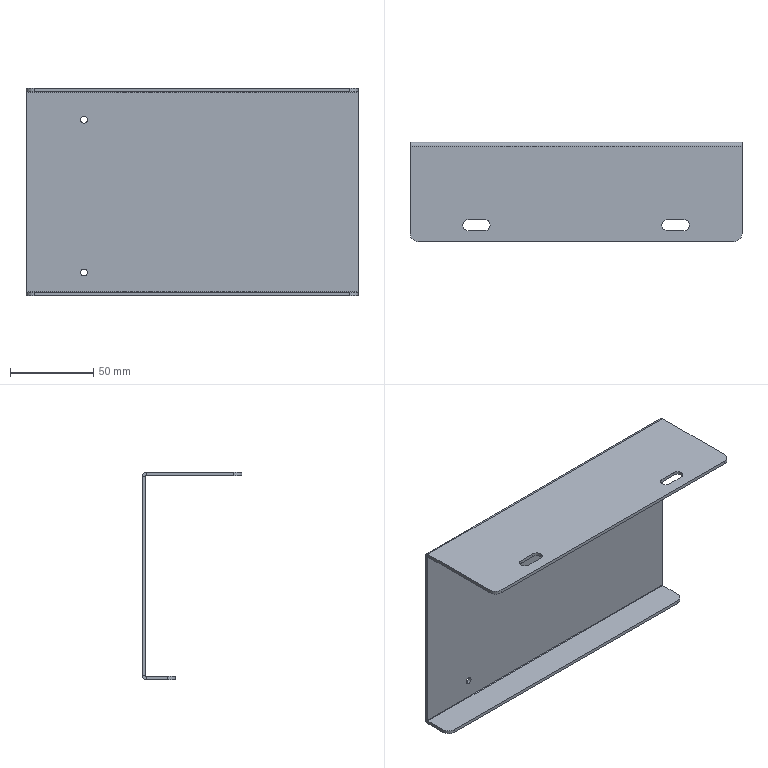Part | SolidWorks | features Fillet 1, FlatPattern 1, HoleWzd 1, ICE 1, SMBaseFlange 1, SheetMetal 1 | 1 solid | 40 faces | box 200 x 60 x 125 mm | volume 79463 mm3 | plane 22 | cylinder 18 | commonest cylinder face diameters 6.5 x6 4.2 x4 10 x4 0.6 x2 4.6 x2
STEP:
#1=CARTESIAN_POINT('',(35.,-2.,-113.1));
#2=VERTEX_POINT('',#1);
#3=CARTESIAN_POINT('',(35.,-2.,-108.9));
#4=VERTEX_POINT('',#3);
#5=CARTESIAN_POINT('',(35.,-2.,-111.));
#6=DIRECTION('',(0.,1.,0.));
#7=DIRECTION('',(0.,0.,1.));
#8=AXIS2_PLACEMENT_3D('',#5,#6,#7);
#9=CIRCLE('',#8,2.1);
#10=EDGE_CURVE('',#2,#4,#9,.T.);
#11=ORIENTED_EDGE('',*,*,#10,.F.);
#12=CARTESIAN_POINT('',(35.,0.,-113.1));
#13=VERTEX_POINT('',#12);
#14=CARTESIAN_POINT('',(35.,0.,-113.1));
#15=DIRECTION('',(0.,1.,0.));
#16=VECTOR('',#15,1000.);
#17=LINE('',#14,#16);
#18=EDGE_CURVE('',#2,#13,#17,.T.);
#19=ORIENTED_EDGE('',*,*,#18,.T.);
#20=CARTESIAN_POINT('',(35.,0.,-108.9));
#21=VERTEX_POINT('',#20);
#22=CARTESIAN_POINT('',(35.,0.,-111.));
#23=DIRECTION('',(0.,1.,0.));
#24=DIRECTION('',(0.,0.,1.));
#25=AXIS2_PLACEMENT_3D('',#22,#23,#24);
#26=CIRCLE('',#25,2.1);
#27=EDGE_CURVE('',#13,#21,#26,.T.);
#28=ORIENTED_EDGE('',*,*,#27,.T.);
#29=CARTESIAN_POINT('',(35.,0.,-108.9));
#30=DIRECTION('',(0.,1.,0.));
#31=VECTOR('',#30,1000.);
#32=LINE('',#29,#31);
#33=EDGE_CURVE('',#4,#21,#32,.T.);
#34=ORIENTED_EDGE('',*,*,#33,.F.);
#35=EDGE_LOOP('',(#11,#19,#28,#34));
#36=FACE_OUTER_BOUND('',#35,.T.);
#37=CARTESIAN_POINT('',(35.,0.,-111.));
#38=DIRECTION('',(0.,1.,0.));
#39=DIRECTION('',(0.,0.,1.));
#40=AXIS2_PLACEMENT_3D('',#37,#38,#39);
#41=CYLINDRICAL_SURFACE('',#40,2.1);
#42=ADVANCED_FACE('',(#36),#41,.F.);
#43=CARTESIAN_POINT('',(35.,-2.,-21.1));
#44=VERTEX_POINT('',#43);
#45=CARTESIAN_POINT('',(35.,-2.,-16.9));
#46=VERTEX_POINT('',#45);
#47=CARTESIAN_POINT('',(35.,-2.,-19.));
#48=DIRECTION('',(0.,1.,0.));
#49=DIRECTION('',(0.,0.,1.));
#50=AXIS2_PLACEMENT_3D('',#47,#48,#49);
#51=CIRCLE('',#50,2.1);
#52=EDGE_CURVE('',#44,#46,#51,.T.);
#53=ORIENTED_EDGE('',*,*,#52,.F.);
#54=CARTESIAN_POINT('',(35.,0.,-21.1));
#55=VERTEX_POINT('',#54);
#56=CARTESIAN_POINT('',(35.,0.,-21.1));
#57=DIRECTION('',(0.,1.,0.));
#58=VECTOR('',#57,1000.);
#59=LINE('',#56,#58);
#60=EDGE_CURVE('',#44,#55,#59,.T.);
#61=ORIENTED_EDGE('',*,*,#60,.T.);
#62=CARTESIAN_POINT('',(35.,0.,-16.9));
#63=VERTEX_POINT('',#62);
#64=CARTESIAN_POINT('',(35.,0.,-19.));
#65=DIRECTION('',(0.,1.,0.));
#66=DIRECTION('',(0.,0.,1.));
#67=AXIS2_PLACEMENT_3D('',#64,#65,#66);
#68=CIRCLE('',#67,2.1);
#69=EDGE_CURVE('',#55,#63,#68,.T.);
#70=ORIENTED_EDGE('',*,*,#69,.T.);
#71=CARTESIAN_POINT('',(35.,0.,-16.9));
#72=DIRECTION('',(0.,1.,0.));
#73=VECTOR('',#72,1000.);
#74=LINE('',#71,#73);
#75=EDGE_CURVE('',#46,#63,#74,.T.);
#76=ORIENTED_EDGE('',*,*,#75,.F.);
#77=EDGE_LOOP('',(#53,#61,#70,#76));
#78=FACE_OUTER_BOUND('',#77,.T.);
#79=CARTESIAN_POINT('',(35.,0.,-19.));
#80=DIRECTION('',(0.,1.,0.));
#81=DIRECTION('',(0.,0.,1.));
#82=AXIS2_PLACEMENT_3D('',#79,#80,#81);
#83=CYLINDRICAL_SURFACE('',#82,2.1);
#84=ADVANCED_FACE('',(#78),#83,.F.);
#85=CARTESIAN_POINT('',(165.,-46.75,-2.));
#86=VERTEX_POINT('',#85);
#87=CARTESIAN_POINT('',(168.25,-50.,-2.));
#88=VERTEX_POINT('',#87);
#89=CARTESIAN_POINT('',(165.,-50.,-2.));
#90=DIRECTION('',(0.,0.,-1.));
#91=DIRECTION('',(0.,-1.,0.));
#92=AXIS2_PLACEMENT_3D('',#89,#90,#91);
#93=CIRCLE('',#92,3.25);
#94=EDGE_CURVE('',#86,#88,#93,.T.);
#95=ORIENTED_EDGE('',*,*,#94,.T.);
#96=CARTESIAN_POINT('',(168.25,-50.,0.));
#97=VERTEX_POINT('',#96);
#98=CARTESIAN_POINT('',(168.25,-50.,-10.));
#99=DIRECTION('',(0.,0.,1.));
#100=VECTOR('',#99,1000.);
#101=LINE('',#98,#100);
#102=EDGE_CURVE('',#88,#97,#101,.T.);
#103=ORIENTED_EDGE('',*,*,#102,.T.);
#104=CARTESIAN_POINT('',(165.,-46.75,0.));
#105=VERTEX_POINT('',#104);
#106=CARTESIAN_POINT('',(165.,-50.,0.));
#107=DIRECTION('',(0.,0.,-1.));
#108=DIRECTION('',(-1.,0.,0.));
#109=AXIS2_PLACEMENT_3D('',#106,#107,#108);
#110=CIRCLE('',#109,3.25);
#111=EDGE_CURVE('',#105,#97,#110,.T.);
#112=ORIENTED_EDGE('',*,*,#111,.F.);
#113=CARTESIAN_POINT('',(165.,-46.75,-10.));
#114=DIRECTION('',(0.,0.,1.));
#115=VECTOR('',#114,1000.);
#116=LINE('',#113,#115);
#117=EDGE_CURVE('',#86,#105,#116,.T.);
#118=ORIENTED_EDGE('',*,*,#117,.F.);
#119=EDGE_LOOP('',(#95,#103,#112,#118));
#120=FACE_OUTER_BOUND('',#119,.T.);
#121=CARTESIAN_POINT('',(165.,-50.,-10.));
#122=DIRECTION('',(0.,0.,1.));
#123=DIRECTION('',(1.,0.,0.));
#124=AXIS2_PLACEMENT_3D('',#121,#122,#123);
#125=CYLINDRICAL_SURFACE('',#124,3.25);
#126=ADVANCED_FACE('',(#120),#125,.F.);
#127=CARTESIAN_POINT('',(45.,-46.75,-2.));
#128=VERTEX_POINT('',#127);
#129=CARTESIAN_POINT('',(48.25,-50.,-2.));
#130=VERTEX_POINT('',#129);
#131=CARTESIAN_POINT('',(45.,-50.,-2.));
#132=DIRECTION('',(0.,0.,-1.));
#133=DIRECTION('',(0.,-1.,0.));
#134=AXIS2_PLACEMENT_3D('',#131,#132,#133);
#135=CIRCLE('',#134,3.25);
#136=EDGE_CURVE('',#128,#130,#135,.T.);
#137=ORIENTED_EDGE('',*,*,#136,.T.);
#138=CARTESIAN_POINT('',(48.25,-50.,0.));
#139=VERTEX_POINT('',#138);
#140=CARTESIAN_POINT('',(48.25,-50.,-10.));
#141=DIRECTION('',(0.,0.,1.));
#142=VECTOR('',#141,1000.);
#143=LINE('',#140,#142);
#144=EDGE_CURVE('',#130,#139,#143,.T.);
#145=ORIENTED_EDGE('',*,*,#144,.T.);
#146=CARTESIAN_POINT('',(45.,-46.75,0.));
#147=VERTEX_POINT('',#146);
#148=CARTESIAN_POINT('',(45.,-50.,0.));
#149=DIRECTION('',(0.,0.,-1.));
#150=DIRECTION('',(-1.,0.,0.));
#151=AXIS2_PLACEMENT_3D('',#148,#149,#150);
#152=CIRCLE('',#151,3.25);
#153=EDGE_CURVE('',#147,#139,#152,.T.);
#154=ORIENTED_EDGE('',*,*,#153,.F.);
#155=CARTESIAN_POINT('',(45.,-46.75,-10.));
#156=DIRECTION('',(0.,0.,1.));
#157=VECTOR('',#156,1000.);
#158=LINE('',#155,#157);
#159=EDGE_CURVE('',#128,#147,#158,.T.);
#160=ORIENTED_EDGE('',*,*,#159,.F.);
#161=EDGE_LOOP('',(#137,#145,#154,#160));
#162=FACE_OUTER_BOUND('',#161,.T.);
#163=CARTESIAN_POINT('',(45.,-50.,-10.));
#164=DIRECTION('',(0.,0.,1.));
#165=DIRECTION('',(1.,0.,0.));
#166=AXIS2_PLACEMENT_3D('',#163,#164,#165);
#167=CYLINDRICAL_SURFACE('',#166,3.25);
#168=ADVANCED_FACE('',(#162),#167,.F.);
#169=CARTESIAN_POINT('',(195.,-60.,0.));
#170=VERTEX_POINT('',#169);
#171=CARTESIAN_POINT('',(5.,-60.,0.));
#172=VERTEX_POINT('',#171);
#173=CARTESIAN_POINT('',(200.,-60.,0.));
#174=DIRECTION('',(-1.,0.,0.));
#175=VECTOR('',#174,1000.);
#176=LINE('',#173,#175);
#177=EDGE_CURVE('',#170,#172,#176,.T.);
#178=ORIENTED_EDGE('',*,*,#177,.F.);
#179=CARTESIAN_POINT('',(200.,-55.,0.));
#180=VERTEX_POINT('',#179);
#181=CARTESIAN_POINT('',(195.,-55.,0.));
#182=DIRECTION('',(0.,0.,1.));
#183=DIRECTION('',(0.,-1.,0.));
#184=AXIS2_PLACEMENT_3D('',#181,#182,#183);
#185=CIRCLE('',#184,5.);
#186=EDGE_CURVE('',#170,#180,#185,.T.);
#187=ORIENTED_EDGE('',*,*,#186,.T.);
#188=CARTESIAN_POINT('',(200.,-2.3,0.));
#189=VERTEX_POINT('',#188);
#190=CARTESIAN_POINT('',(200.,0.,0.));
#191=DIRECTION('',(0.,1.,0.));
#192=VECTOR('',#191,1000.);
#193=LINE('',#190,#192);
#194=EDGE_CURVE('',#180,#189,#193,.T.);
#195=ORIENTED_EDGE('',*,*,#194,.T.);
#196=CARTESIAN_POINT('',(0.,-2.3,0.));
#197=VERTEX_POINT('',#196);
#198=CARTESIAN_POINT('',(200.,-2.3,0.));
#199=DIRECTION('',(-1.,0.,0.));
#200=VECTOR('',#199,1000.);
#201=LINE('',#198,#200);
#202=EDGE_CURVE('',#189,#197,#201,.T.);
#203=ORIENTED_EDGE('',*,*,#202,.T.);
#204=CARTESIAN_POINT('',(0.,-55.,0.));
#205=VERTEX_POINT('',#204);
#206=CARTESIAN_POINT('',(0.,0.,0.));
#207=DIRECTION('',(0.,1.,0.));
#208=VECTOR('',#207,1000.);
#209=LINE('',#206,#208);
#210=EDGE_CURVE('',#205,#197,#209,.T.);
#211=ORIENTED_EDGE('',*,*,#210,.F.);
#212=CARTESIAN_POINT('',(5.,-55.,0.));
#213=DIRECTION('',(0.,0.,1.));
#214=DIRECTION('',(0.,-1.,0.));
#215=AXIS2_PLACEMENT_3D('',#212,#213,#214);
#216=CIRCLE('',#215,5.);
#217=EDGE_CURVE('',#205,#172,#216,.T.);
#218=ORIENTED_EDGE('',*,*,#217,.T.);
#219=EDGE_LOOP('',(#178,#187,#195,#203,#211,#218));
#220=FACE_OUTER_BOUND('',#219,.T.);
#221=CARTESIAN_POINT('',(35.,-46.75,0.));
#222=VERTEX_POINT('',#221);
#223=CARTESIAN_POINT('',(45.,-46.75,0.));
#224=DIRECTION('',(1.,0.,0.));
#225=VECTOR('',#224,1000.);
#226=LINE('',#223,#225);
#227=EDGE_CURVE('',#222,#147,#226,.T.);
#228=ORIENTED_EDGE('',*,*,#227,.T.);
#229=ORIENTED_EDGE('',*,*,#153,.T.);
#230=CARTESIAN_POINT('',(45.,-53.25,0.));
#231=VERTEX_POINT('',#230);
#232=CARTESIAN_POINT('',(45.,-50.,0.));
#233=DIRECTION('',(0.,0.,-1.));
#234=DIRECTION('',(-1.,0.,0.));
#235=AXIS2_PLACEMENT_3D('',#232,#233,#234);
#236=CIRCLE('',#235,3.25);
#237=EDGE_CURVE('',#139,#231,#236,.T.);
#238=ORIENTED_EDGE('',*,*,#237,.T.);
#239=CARTESIAN_POINT('',(35.,-53.25,0.));
#240=VERTEX_POINT('',#239);
#241=CARTESIAN_POINT('',(45.,-53.25,0.));
#242=DIRECTION('',(-1.,0.,0.));
#243=VECTOR('',#242,1000.);
#244=LINE('',#241,#243);
#245=EDGE_CURVE('',#231,#240,#244,.T.);
#246=ORIENTED_EDGE('',*,*,#245,.T.);
#247=CARTESIAN_POINT('',(35.,-50.,0.));
#248=DIRECTION('',(0.,0.,-1.));
#249=DIRECTION('',(-1.,0.,0.));
#250=AXIS2_PLACEMENT_3D('',#247,#248,#249);
#251=CIRCLE('',#250,3.25);
#252=EDGE_CURVE('',#240,#222,#251,.T.);
#253=ORIENTED_EDGE('',*,*,#252,.T.);
#254=EDGE_LOOP('',(#228,#229,#238,#246,#253));
#255=FACE_BOUND('',#254,.T.);
#256=CARTESIAN_POINT('',(155.,-46.75,0.));
#257=VERTEX_POINT('',#256);
#258=CARTESIAN_POINT('',(165.,-46.75,0.));
#259=DIRECTION('',(1.,0.,0.));
#260=VECTOR('',#259,1000.);
#261=LINE('',#258,#260);
#262=EDGE_CURVE('',#257,#105,#261,.T.);
#263=ORIENTED_EDGE('',*,*,#262,.T.);
#264=ORIENTED_EDGE('',*,*,#111,.T.);
#265=CARTESIAN_POINT('',(165.,-53.25,0.));
#266=VERTEX_POINT('',#265);
#267=CARTESIAN_POINT('',(165.,-50.,0.));
#268=DIRECTION('',(0.,0.,-1.));
#269=DIRECTION('',(-1.,0.,0.));
#270=AXIS2_PLACEMENT_3D('',#267,#268,#269);
#271=CIRCLE('',#270,3.25);
#272=EDGE_CURVE('',#97,#266,#271,.T.);
#273=ORIENTED_EDGE('',*,*,#272,.T.);
#274=CARTESIAN_POINT('',(155.,-53.25,0.));
#275=VERTEX_POINT('',#274);
#276=CARTESIAN_POINT('',(165.,-53.25,0.));
#277=DIRECTION('',(-1.,0.,0.));
#278=VECTOR('',#277,1000.);
#279=LINE('',#276,#278);
#280=EDGE_CURVE('',#266,#275,#279,.T.);
#281=ORIENTED_EDGE('',*,*,#280,.T.);
#282=CARTESIAN_POINT('',(155.,-50.,0.));
#283=DIRECTION('',(0.,0.,-1.));
#284=DIRECTION('',(-1.,0.,0.));
#285=AXIS2_PLACEMENT_3D('',#282,#283,#284);
#286=CIRCLE('',#285,3.25);
#287=EDGE_CURVE('',#275,#257,#286,.T.);
#288=ORIENTED_EDGE('',*,*,#287,.T.);
#289=EDGE_LOOP('',(#263,#264,#273,#281,#288));
#290=FACE_BOUND('',#289,.T.);
#291=CARTESIAN_POINT('',(200.,0.,0.));
#292=DIRECTION('',(0.,0.,1.));
#293=DIRECTION('',(0.,-1.,0.));
#294=AXIS2_PLACEMENT_3D('',#291,#292,#293);
#295=PLANE('',#294);
#296=ADVANCED_FACE('',(#220,#255,#290),#295,.T.);
#297=ORIENTED_EDGE('',*,*,#136,.F.);
#298=CARTESIAN_POINT('',(35.,-46.75,-2.));
#299=VERTEX_POINT('',#298);
#300=CARTESIAN_POINT('',(200.,-46.75,-2.));
#301=DIRECTION('',(1.,0.,0.));
#302=VECTOR('',#301,1000.);
#303=LINE('',#300,#302);
#304=EDGE_CURVE('',#299,#128,#303,.T.);
#305=ORIENTED_EDGE('',*,*,#304,.F.);
#306=CARTESIAN_POINT('',(35.,-53.25,-2.));
#307=VERTEX_POINT('',#306);
#308=CARTESIAN_POINT('',(35.,-50.,-2.));
#309=DIRECTION('',(0.,0.,-1.));
#310=DIRECTION('',(0.,-1.,0.));
#311=AXIS2_PLACEMENT_3D('',#308,#309,#310);
#312=CIRCLE('',#311,3.25);
#313=EDGE_CURVE('',#307,#299,#312,.T.);
#314=ORIENTED_EDGE('',*,*,#313,.F.);
#315=CARTESIAN_POINT('',(45.,-53.25,-2.));
#316=VERTEX_POINT('',#315);
#317=CARTESIAN_POINT('',(200.,-53.25,-2.));
#318=DIRECTION('',(-1.,0.,0.));
#319=VECTOR('',#318,1000.);
#320=LINE('',#317,#319);
#321=EDGE_CURVE('',#316,#307,#320,.T.);
#322=ORIENTED_EDGE('',*,*,#321,.F.);
#323=CARTESIAN_POINT('',(45.,-50.,-2.));
#324=DIRECTION('',(0.,0.,-1.));
#325=DIRECTION('',(0.,-1.,0.));
#326=AXIS2_PLACEMENT_3D('',#323,#324,#325);
#327=CIRCLE('',#326,3.25);
#328=EDGE_CURVE('',#130,#316,#327,.T.);
#329=ORIENTED_EDGE('',*,*,#328,.F.);
#330=EDGE_LOOP('',(#297,#305,#314,#322,#329));
#331=FACE_BOUND('',#330,.T.);
#332=CARTESIAN_POINT('',(200.,-55.,-2.));
#333=VERTEX_POINT('',#332);
#334=CARTESIAN_POINT('',(200.,-2.3,-2.));
#335=VERTEX_POINT('',#334);
#336=CARTESIAN_POINT('',(200.,0.,-2.));
#337=DIRECTION('',(0.,1.,0.));
#338=VECTOR('',#337,1000.);
#339=LINE('',#336,#338);
#340=EDGE_CURVE('',#333,#335,#339,.T.);
#341=ORIENTED_EDGE('',*,*,#340,.F.);
#342=CARTESIAN_POINT('',(195.,-60.,-2.));
#343=VERTEX_POINT('',#342);
#344=CARTESIAN_POINT('',(195.,-55.,-2.));
#345=DIRECTION('',(0.,0.,-1.));
#346=DIRECTION('',(0.,-1.,0.));
#347=AXIS2_PLACEMENT_3D('',#344,#345,#346);
#348=CIRCLE('',#347,5.);
#349=EDGE_CURVE('',#333,#343,#348,.T.);
#350=ORIENTED_EDGE('',*,*,#349,.T.);
#351=CARTESIAN_POINT('',(5.,-60.,-2.));
#352=VERTEX_POINT('',#351);
#353=CARTESIAN_POINT('',(200.,-60.,-2.));
#354=DIRECTION('',(-1.,0.,0.));
#355=VECTOR('',#354,1000.);
#356=LINE('',#353,#355);
#357=EDGE_CURVE('',#343,#352,#356,.T.);
#358=ORIENTED_EDGE('',*,*,#357,.T.);
#359=CARTESIAN_POINT('',(0.,-55.,-2.));
#360=VERTEX_POINT('',#359);
#361=CARTESIAN_POINT('',(5.,-55.,-2.));
#362=DIRECTION('',(0.,0.,-1.));
#363=DIRECTION('',(0.,-1.,0.));
#364=AXIS2_PLACEMENT_3D('',#361,#362,#363);
#365=CIRCLE('',#364,5.);
#366=EDGE_CURVE('',#352,#360,#365,.T.);
#367=ORIENTED_EDGE('',*,*,#366,.T.);
#368=CARTESIAN_POINT('',(0.,-2.3,-2.));
#369=VERTEX_POINT('',#368);
#370=CARTESIAN_POINT('',(0.,0.,-2.));
#371=DIRECTION('',(0.,1.,0.));
#372=VECTOR('',#371,1000.);
#373=LINE('',#370,#372);
#374=EDGE_CURVE('',#360,#369,#373,.T.);
#375=ORIENTED_EDGE('',*,*,#374,.T.);
#376=CARTESIAN_POINT('',(200.,-2.3,-2.));
#377=DIRECTION('',(-1.,0.,0.));
#378=VECTOR('',#377,1000.);
#379=LINE('',#376,#378);
#380=EDGE_CURVE('',#335,#369,#379,.T.);
#381=ORIENTED_EDGE('',*,*,#380,.F.);
#382=EDGE_LOOP('',(#341,#350,#358,#367,#375,#381));
#383=FACE_OUTER_BOUND('',#382,.T.);
#384=ORIENTED_EDGE('',*,*,#94,.F.);
#385=CARTESIAN_POINT('',(155.,-46.75,-2.));
#386=VERTEX_POINT('',#385);
#387=CARTESIAN_POINT('',(200.,-46.75,-2.));
#388=DIRECTION('',(1.,0.,0.));
#389=VECTOR('',#388,1000.);
#390=LINE('',#387,#389);
#391=EDGE_CURVE('',#386,#86,#390,.T.);
#392=ORIENTED_EDGE('',*,*,#391,.F.);
#393=CARTESIAN_POINT('',(155.,-53.25,-2.));
#394=VERTEX_POINT('',#393);
#395=CARTESIAN_POINT('',(155.,-50.,-2.));
#396=DIRECTION('',(0.,0.,-1.));
#397=DIRECTION('',(0.,-1.,0.));
#398=AXIS2_PLACEMENT_3D('',#395,#396,#397);
#399=CIRCLE('',#398,3.25);
#400=EDGE_CURVE('',#394,#386,#399,.T.);
#401=ORIENTED_EDGE('',*,*,#400,.F.);
#402=CARTESIAN_POINT('',(165.,-53.25,-2.));
#403=VERTEX_POINT('',#402);
#404=CARTESIAN_POINT('',(200.,-53.25,-2.));
#405=DIRECTION('',(-1.,0.,0.));
#406=VECTOR('',#405,1000.);
#407=LINE('',#404,#406);
#408=EDGE_CURVE('',#403,#394,#407,.T.);
#409=ORIENTED_EDGE('',*,*,#408,.F.);
#410=CARTESIAN_POINT('',(165.,-50.,-2.));
#411=DIRECTION('',(0.,0.,-1.));
#412=DIRECTION('',(0.,-1.,0.));
#413=AXIS2_PLACEMENT_3D('',#410,#411,#412);
#414=CIRCLE('',#413,3.25);
#415=EDGE_CURVE('',#88,#403,#414,.T.);
#416=ORIENTED_EDGE('',*,*,#415,.F.);
#417=EDGE_LOOP('',(#384,#392,#401,#409,#416));
#418=FACE_BOUND('',#417,.T.);
#419=CARTESIAN_POINT('',(200.,0.,-2.));
#420=DIRECTION('',(0.,0.,1.));
#421=DIRECTION('',(0.,-1.,0.));
#422=AXIS2_PLACEMENT_3D('',#419,#420,#421);
#423=PLANE('',#422);
#424=ADVANCED_FACE('',(#331,#383,#418),#423,.F.);
#425=CARTESIAN_POINT('',(200.,0.,-2.3));
#426=VERTEX_POINT('',#425);
#427=CARTESIAN_POINT('',(200.,-2.,-2.3));
#428=VERTEX_POINT('',#427);
#429=CARTESIAN_POINT('',(200.,0.,-2.3));
#430=DIRECTION('',(0.,-1.,0.));
#431=VECTOR('',#430,1000.);
#432=LINE('',#429,#431);
#433=EDGE_CURVE('',#426,#428,#432,.T.);
#434=ORIENTED_EDGE('',*,*,#433,.F.);
#435=CARTESIAN_POINT('',(200.,-2.3,-2.3));
#436=DIRECTION('',(-1.,0.,0.));
#437=DIRECTION('',(0.,0.,-1.));
#438=AXIS2_PLACEMENT_3D('',#435,#436,#437);
#439=CIRCLE('',#438,2.3);
#440=EDGE_CURVE('',#189,#426,#439,.T.);
#441=ORIENTED_EDGE('',*,*,#440,.F.);
#442=CARTESIAN_POINT('',(200.,-2.3,-2.));
#443=DIRECTION('',(0.,0.,1.));
#444=VECTOR('',#443,1000.);
#445=LINE('',#442,#444);
#446=EDGE_CURVE('',#335,#189,#445,.T.);
#447=ORIENTED_EDGE('',*,*,#446,.F.);
#448=CARTESIAN_POINT('',(200.,-2.3,-2.3));
#449=DIRECTION('',(-1.,0.,0.));
#450=DIRECTION('',(0.,0.,-1.));
#451=AXIS2_PLACEMENT_3D('',#448,#449,#450);
#452=CIRCLE('',#451,0.3);
#453=EDGE_CURVE('',#335,#428,#452,.T.);
#454=ORIENTED_EDGE('',*,*,#453,.T.);
#455=EDGE_LOOP('',(#434,#441,#447,#454));
#456=FACE_OUTER_BOUND('',#455,.T.);
#457=CARTESIAN_POINT('',(200.,0.,-2.3));
#458=DIRECTION('',(1.,0.,0.));
#459=DIRECTION('',(0.,0.,-1.));
#460=AXIS2_PLACEMENT_3D('',#457,#458,#459);
#461=PLANE('',#460);
#462=ADVANCED_FACE('',(#456),#461,.T.);
#463=CARTESIAN_POINT('',(200.,0.,-122.7));
#464=VERTEX_POINT('',#463);
#465=CARTESIAN_POINT('',(200.,0.,0.));
#466=DIRECTION('',(0.,0.,-1.));
#467=VECTOR('',#466,1000.);
#468=LINE('',#465,#467);
#469=EDGE_CURVE('',#426,#464,#468,.T.);
#470=ORIENTED_EDGE('',*,*,#469,.F.);
#471=ORIENTED_EDGE('',*,*,#433,.T.);
#472=CARTESIAN_POINT('',(200.,-2.,-122.7));
#473=VERTEX_POINT('',#472);
#474=CARTESIAN_POINT('',(200.,-2.,0.));
#475=DIRECTION('',(0.,0.,-1.));
#476=VECTOR('',#475,1000.);
#477=LINE('',#474,#476);
#478=EDGE_CURVE('',#428,#473,#477,.T.);
#479=ORIENTED_EDGE('',*,*,#478,.T.);
#480=CARTESIAN_POINT('',(200.,-2.,-122.7));
#481=DIRECTION('',(0.,1.,0.));
#482=VECTOR('',#481,1000.);
#483=LINE('',#480,#482);
#484=EDGE_CURVE('',#473,#464,#483,.T.);
#485=ORIENTED_EDGE('',*,*,#484,.T.);
#486=EDGE_LOOP('',(#470,#471,#479,#485));
#487=FACE_OUTER_BOUND('',#486,.T.);
#488=CARTESIAN_POINT('',(200.,-2.3,-2.));
#489=DIRECTION('',(1.,0.,0.));
#490=DIRECTION('',(0.,0.,-1.));
#491=AXIS2_PLACEMENT_3D('',#488,#489,#490);
#492=PLANE('',#491);
#493=ADVANCED_FACE('',(#487),#492,.T.);
#494=CARTESIAN_POINT('',(0.,-2.3,0.));
#495=DIRECTION('',(0.,0.,-1.));
#496=VECTOR('',#495,1000.);
#497=LINE('',#494,#496);
#498=EDGE_CURVE('',#197,#369,#497,.T.);
#499=ORIENTED_EDGE('',*,*,#498,.F.);
#500=CARTESIAN_POINT('',(0.,0.,-2.3));
#501=VERTEX_POINT('',#500);
#502=CARTESIAN_POINT('',(0.,-2.3,-2.3));
#503=DIRECTION('',(-1.,0.,0.));
#504=DIRECTION('',(0.,0.,-1.));
#505=AXIS2_PLACEMENT_3D('',#502,#503,#504);
#506=CIRCLE('',#505,2.3);
#507=EDGE_CURVE('',#197,#501,#506,.T.);
#508=ORIENTED_EDGE('',*,*,#507,.T.);
#509=CARTESIAN_POINT('',(0.,-2.,-2.3));
#510=VERTEX_POINT('',#509);
#511=CARTESIAN_POINT('',(0.,-2.,-2.3));
#512=DIRECTION('',(0.,1.,0.));
#513=VECTOR('',#512,1000.);
#514=LINE('',#511,#513);
#515=EDGE_CURVE('',#510,#501,#514,.T.);
#516=ORIENTED_EDGE('',*,*,#515,.F.);
#517=CARTESIAN_POINT('',(0.,-2.3,-2.3));
#518=DIRECTION('',(-1.,0.,0.));
#519=DIRECTION('',(0.,0.,-1.));
#520=AXIS2_PLACEMENT_3D('',#517,#518,#519);
#521=CIRCLE('',#520,0.3);
#522=EDGE_CURVE('',#369,#510,#521,.T.);
#523=ORIENTED_EDGE('',*,*,#522,.F.);
#524=EDGE_LOOP('',(#499,#508,#516,#523));
#525=FACE_OUTER_BOUND('',#524,.T.);
#526=CARTESIAN_POINT('',(0.,-2.3,0.));
#527=DIRECTION('',(-1.,0.,0.));
#528=DIRECTION('',(0.,0.,1.));
#529=AXIS2_PLACEMENT_3D('',#526,#527,#528);
#530=PLANE('',#529);
#531=ADVANCED_FACE('',(#525),#530,.T.);
#532=ORIENTED_EDGE('',*,*,#374,.F.);
#533=CARTESIAN_POINT('',(0.,-55.,-2.3));
#534=DIRECTION('',(0.,0.,1.));
#535=VECTOR('',#534,1000.);
#536=LINE('',#533,#535);
#537=EDGE_CURVE('',#360,#205,#536,.T.);
#538=ORIENTED_EDGE('',*,*,#537,.T.);
#539=ORIENTED_EDGE('',*,*,#210,.T.);
#540=ORIENTED_EDGE('',*,*,#498,.T.);
#541=EDGE_LOOP('',(#532,#538,#539,#540));
#542=FACE_OUTER_BOUND('',#541,.T.);
#543=CARTESIAN_POINT('',(0.,-2.,-2.3));
#544=DIRECTION('',(-1.,0.,0.));
#545=DIRECTION('',(0.,0.,1.));
#546=AXIS2_PLACEMENT_3D('',#543,#544,#545);
#547=PLANE('',#546);
#548=ADVANCED_FACE('',(#542),#547,.T.);
#549=CARTESIAN_POINT('',(200.,-2.3,-125.));
#550=VERTEX_POINT('',#549);
#551=CARTESIAN_POINT('',(200.,-2.3,-123.));
#552=VERTEX_POINT('',#551);
#553=CARTESIAN_POINT('',(200.,-2.3,-125.));
#554=DIRECTION('',(0.,0.,1.));
#555=VECTOR('',#554,1000.);
#556=LINE('',#553,#555);
#557=EDGE_CURVE('',#550,#552,#556,.T.);
#558=ORIENTED_EDGE('',*,*,#557,.F.);
#559=CARTESIAN_POINT('',(200.,-2.3,-122.7));
#560=DIRECTION('',(-1.,0.,0.));
#561=DIRECTION('',(0.,0.,-1.));
#562=AXIS2_PLACEMENT_3D('',#559,#560,#561);
#563=CIRCLE('',#562,2.3);
#564=EDGE_CURVE('',#464,#550,#563,.T.);
#565=ORIENTED_EDGE('',*,*,#564,.F.);
#566=ORIENTED_EDGE('',*,*,#484,.F.);
#567=CARTESIAN_POINT('',(200.,-2.3,-122.7));
#568=DIRECTION('',(-1.,0.,0.));
#569=DIRECTION('',(0.,0.,-1.));
#570=AXIS2_PLACEMENT_3D('',#567,#568,#569);
#571=CIRCLE('',#570,0.3);
#572=EDGE_CURVE('',#473,#552,#571,.T.);
#573=ORIENTED_EDGE('',*,*,#572,.T.);
#574=EDGE_LOOP('',(#558,#565,#566,#573));
#575=FACE_OUTER_BOUND('',#574,.T.);
#576=CARTESIAN_POINT('',(200.,-2.3,-125.));
#577=DIRECTION('',(1.,0.,0.));
#578=DIRECTION('',(0.,0.,-1.));
#579=AXIS2_PLACEMENT_3D('',#576,#577,#578);
#580=PLANE('',#579);
#581=ADVANCED_FACE('',(#575),#580,.T.);
#582=CARTESIAN_POINT('',(200.,-15.,-123.));
#583=VERTEX_POINT('',#582);
#584=CARTESIAN_POINT('',(200.,0.,-123.));
#585=DIRECTION('',(0.,-1.,0.));
#586=VECTOR('',#585,1000.);
#587=LINE('',#584,#586);
#588=EDGE_CURVE('',#552,#583,#587,.T.);
#589=ORIENTED_EDGE('',*,*,#588,.T.);
#590=CARTESIAN_POINT('',(200.,-15.,-125.));
#591=VERTEX_POINT('',#590);
#592=CARTESIAN_POINT('',(200.,-15.,-122.7));
#593=DIRECTION('',(0.,0.,-1.));
#594=VECTOR('',#593,1000.);
#595=LINE('',#592,#594);
#596=EDGE_CURVE('',#583,#591,#595,.T.);
#597=ORIENTED_EDGE('',*,*,#596,.T.);
#598=CARTESIAN_POINT('',(200.,0.,-125.));
#599=DIRECTION('',(0.,-1.,0.));
#600=VECTOR('',#599,1000.);
#601=LINE('',#598,#600);
#602=EDGE_CURVE('',#550,#591,#601,.T.);
#603=ORIENTED_EDGE('',*,*,#602,.F.);
#604=ORIENTED_EDGE('',*,*,#557,.T.);
#605=EDGE_LOOP('',(#589,#597,#603,#604));
#606=FACE_OUTER_BOUND('',#605,.T.);
#607=CARTESIAN_POINT('',(200.,-2.,-122.7));
#608=DIRECTION('',(1.,0.,0.));
#609=DIRECTION('',(0.,0.,-1.));
#610=AXIS2_PLACEMENT_3D('',#607,#608,#609);
#611=PLANE('',#610);
#612=ADVANCED_FACE('',(#606),#611,.T.);
#613=CARTESIAN_POINT('',(0.,0.,-122.7));
#614=VERTEX_POINT('',#613);
#615=CARTESIAN_POINT('',(0.,-2.,-122.7));
#616=VERTEX_POINT('',#615);
#617=CARTESIAN_POINT('',(0.,0.,-122.7));
#618=DIRECTION('',(0.,-1.,0.));
#619=VECTOR('',#618,1000.);
#620=LINE('',#617,#619);
#621=EDGE_CURVE('',#614,#616,#620,.T.);
#622=ORIENTED_EDGE('',*,*,#621,.F.);
#623=CARTESIAN_POINT('',(0.,-2.3,-125.));
#624=VERTEX_POINT('',#623);
#625=CARTESIAN_POINT('',(0.,-2.3,-122.7));
#626=DIRECTION('',(-1.,0.,0.));
#627=DIRECTION('',(0.,0.,-1.));
#628=AXIS2_PLACEMENT_3D('',#625,#626,#627);
#629=CIRCLE('',#628,2.3);
#630=EDGE_CURVE('',#614,#624,#629,.T.);
#631=ORIENTED_EDGE('',*,*,#630,.T.);
#632=CARTESIAN_POINT('',(0.,-2.3,-123.));
#633=VERTEX_POINT('',#632);
#634=CARTESIAN_POINT('',(0.,-2.3,-123.));
#635=DIRECTION('',(0.,0.,-1.));
#636=VECTOR('',#635,1000.);
#637=LINE('',#634,#636);
#638=EDGE_CURVE('',#633,#624,#637,.T.);
#639=ORIENTED_EDGE('',*,*,#638,.F.);
#640=CARTESIAN_POINT('',(0.,-2.3,-122.7));
#641=DIRECTION('',(-1.,0.,0.));
#642=DIRECTION('',(0.,0.,-1.));
#643=AXIS2_PLACEMENT_3D('',#640,#641,#642);
#644=CIRCLE('',#643,0.3);
#645=EDGE_CURVE('',#616,#633,#644,.T.);
#646=ORIENTED_EDGE('',*,*,#645,.F.);
#647=EDGE_LOOP('',(#622,#631,#639,#646));
#648=FACE_OUTER_BOUND('',#647,.T.);
#649=CARTESIAN_POINT('',(0.,0.,-122.7));
#650=DIRECTION('',(-1.,0.,0.));
#651=DIRECTION('',(0.,0.,1.));
#652=AXIS2_PLACEMENT_3D('',#649,#650,#651);
#653=PLANE('',#652);
#654=ADVANCED_FACE('',(#648),#653,.T.);
#655=CARTESIAN_POINT('',(0.,0.,0.));
#656=DIRECTION('',(0.,0.,-1.));
#657=VECTOR('',#656,1000.);
#658=LINE('',#655,#657);
#659=EDGE_CURVE('',#501,#614,#658,.T.);
#660=ORIENTED_EDGE('',*,*,#659,.T.);
#661=ORIENTED_EDGE('',*,*,#621,.T.);
#662=CARTESIAN_POINT('',(0.,-2.,0.));
#663=DIRECTION('',(0.,0.,-1.));
#664=VECTOR('',#663,1000.);
#665=LINE('',#662,#664);
#666=EDGE_CURVE('',#510,#616,#665,.T.);
#667=ORIENTED_EDGE('',*,*,#666,.F.);
#668=ORIENTED_EDGE('',*,*,#515,.T.);
#669=EDGE_LOOP('',(#660,#661,#667,#668));
#670=FACE_OUTER_BOUND('',#669,.T.);
#671=CARTESIAN_POINT('',(0.,-2.3,-123.));
#672=DIRECTION('',(-1.,0.,0.));
#673=DIRECTION('',(0.,0.,1.));
#674=AXIS2_PLACEMENT_3D('',#671,#672,#673);
#675=PLANE('',#674);
#676=ADVANCED_FACE('',(#670),#675,.T.);
#677=CARTESIAN_POINT('',(0.,-15.,-123.));
#678=VERTEX_POINT('',#677);
#679=CARTESIAN_POINT('',(0.,0.,-123.));
#680=DIRECTION('',(0.,-1.,0.));
#681=VECTOR('',#680,1000.);
#682=LINE('',#679,#681);
#683=EDGE_CURVE('',#633,#678,#682,.T.);
#684=ORIENTED_EDGE('',*,*,#683,.T.);
#685=CARTESIAN_POINT('',(5.,-20.,-123.));
#686=VERTEX_POINT('',#685);
#687=CARTESIAN_POINT('',(5.,-15.,-123.));
#688=DIRECTION('',(0.,0.,1.));
#689=DIRECTION('',(-1.,0.,0.));
#690=AXIS2_PLACEMENT_3D('',#687,#688,#689);
#691=CIRCLE('',#690,5.);
#692=EDGE_CURVE('',#678,#686,#691,.T.);
#693=ORIENTED_EDGE('',*,*,#692,.T.);
#694=CARTESIAN_POINT('',(195.,-20.,-123.));
#695=VERTEX_POINT('',#694);
#696=CARTESIAN_POINT('',(200.,-20.,-123.));
#697=DIRECTION('',(-1.,0.,0.));
#698=VECTOR('',#697,1000.);
#699=LINE('',#696,#698);
#700=EDGE_CURVE('',#695,#686,#699,.T.);
#701=ORIENTED_EDGE('',*,*,#700,.F.);
#702=CARTESIAN_POINT('',(195.,-15.,-123.));
#703=DIRECTION('',(0.,0.,1.));
#704=DIRECTION('',(-1.,0.,0.));
#705=AXIS2_PLACEMENT_3D('',#702,#703,#704);
#706=CIRCLE('',#705,5.);
#707=EDGE_CURVE('',#695,#583,#706,.T.);
#708=ORIENTED_EDGE('',*,*,#707,.T.);
#709=ORIENTED_EDGE('',*,*,#588,.F.);
#710=CARTESIAN_POINT('',(200.,-2.3,-123.));
#711=DIRECTION('',(-1.,0.,0.));
#712=VECTOR('',#711,1000.);
#713=LINE('',#710,#712);
#714=EDGE_CURVE('',#552,#633,#713,.T.);
#715=ORIENTED_EDGE('',*,*,#714,.T.);
#716=EDGE_LOOP('',(#684,#693,#701,#708,#709,#715));
#717=FACE_OUTER_BOUND('',#716,.T.);
#718=CARTESIAN_POINT('',(200.,0.,-123.));
#719=DIRECTION('',(0.,0.,-1.));
#720=DIRECTION('',(-1.,0.,0.));
#721=AXIS2_PLACEMENT_3D('',#718,#719,#720);
#722=PLANE('',#721);
#723=ADVANCED_FACE('',(#717),#722,.F.);
#724=ORIENTED_EDGE('',*,*,#700,.T.);
#725=CARTESIAN_POINT('',(5.,-20.,-125.));
#726=VERTEX_POINT('',#725);
#727=CARTESIAN_POINT('',(5.,-20.,-125.));
#728=DIRECTION('',(0.,0.,-1.));
#729=VECTOR('',#728,1000.);
#730=LINE('',#727,#729);
#731=EDGE_CURVE('',#686,#726,#730,.T.);
#732=ORIENTED_EDGE('',*,*,#731,.T.);
#733=CARTESIAN_POINT('',(195.,-20.,-125.));
#734=VERTEX_POINT('',#733);
#735=CARTESIAN_POINT('',(200.,-20.,-125.));
#736=DIRECTION('',(-1.,0.,0.));
#737=VECTOR('',#736,1000.);
#738=LINE('',#735,#737);
#739=EDGE_CURVE('',#734,#726,#738,.T.);
#740=ORIENTED_EDGE('',*,*,#739,.F.);
#741=CARTESIAN_POINT('',(195.,-20.,-125.));
#742=DIRECTION('',(0.,0.,1.));
#743=VECTOR('',#742,1000.);
#744=LINE('',#741,#743);
#745=EDGE_CURVE('',#734,#695,#744,.T.);
#746=ORIENTED_EDGE('',*,*,#745,.T.);
#747=EDGE_LOOP('',(#724,#732,#740,#746));
#748=FACE_OUTER_BOUND('',#747,.T.);
#749=CARTESIAN_POINT('',(200.,-20.,-125.));
#750=DIRECTION('',(0.,-1.,0.));
#751=DIRECTION('',(0.,0.,-1.));
#752=AXIS2_PLACEMENT_3D('',#749,#750,#751);
#753=PLANE('',#752);
#754=ADVANCED_FACE('',(#748),#753,.T.);
#755=ORIENTED_EDGE('',*,*,#739,.T.);
#756=CARTESIAN_POINT('',(0.,-15.,-125.));
#757=VERTEX_POINT('',#756);
#758=CARTESIAN_POINT('',(5.,-15.,-125.));
#759=DIRECTION('',(0.,0.,-1.));
#760=DIRECTION('',(-1.,0.,0.));
#761=AXIS2_PLACEMENT_3D('',#758,#759,#760);
#762=CIRCLE('',#761,5.);
#763=EDGE_CURVE('',#726,#757,#762,.T.);
#764=ORIENTED_EDGE('',*,*,#763,.T.);
#765=CARTESIAN_POINT('',(0.,0.,-125.));
#766=DIRECTION('',(0.,-1.,0.));
#767=VECTOR('',#766,1000.);
#768=LINE('',#765,#767);
#769=EDGE_CURVE('',#624,#757,#768,.T.);
#770=ORIENTED_EDGE('',*,*,#769,.F.);
#771=CARTESIAN_POINT('',(200.,-2.3,-125.));
#772=DIRECTION('',(-1.,0.,0.));
#773=VECTOR('',#772,1000.);
#774=LINE('',#771,#773);
#775=EDGE_CURVE('',#550,#624,#774,.T.);
#776=ORIENTED_EDGE('',*,*,#775,.F.);
#777=ORIENTED_EDGE('',*,*,#602,.T.);
#778=CARTESIAN_POINT('',(195.,-15.,-125.));
#779=DIRECTION('',(0.,0.,-1.));
#780=DIRECTION('',(-1.,0.,0.));
#781=AXIS2_PLACEMENT_3D('',#778,#779,#780);
#782=CIRCLE('',#781,5.);
#783=EDGE_CURVE('',#591,#734,#782,.T.);
#784=ORIENTED_EDGE('',*,*,#783,.T.);
#785=EDGE_LOOP('',(#755,#764,#770,#776,#777,#784));
#786=FACE_OUTER_BOUND('',#785,.T.);
#787=CARTESIAN_POINT('',(200.,0.,-125.));
#788=DIRECTION('',(0.,0.,-1.));
#789=DIRECTION('',(-1.,0.,0.));
#790=AXIS2_PLACEMENT_3D('',#787,#788,#789);
#791=PLANE('',#790);
#792=ADVANCED_FACE('',(#786),#791,.T.);
#793=ORIENTED_EDGE('',*,*,#630,.F.);
#794=CARTESIAN_POINT('',(200.,0.,-122.7));
#795=DIRECTION('',(-1.,0.,0.));
#796=VECTOR('',#795,1000.);
#797=LINE('',#794,#796);
#798=EDGE_CURVE('',#464,#614,#797,.T.);
#799=ORIENTED_EDGE('',*,*,#798,.F.);
#800=ORIENTED_EDGE('',*,*,#564,.T.);
#801=ORIENTED_EDGE('',*,*,#775,.T.);
#802=EDGE_LOOP('',(#793,#799,#800,#801));
#803=FACE_OUTER_BOUND('',#802,.T.);
#804=CARTESIAN_POINT('',(200.,-2.3,-122.7));
#805=DIRECTION('',(-1.,0.,0.));
#806=DIRECTION('',(0.,0.,1.));
#807=AXIS2_PLACEMENT_3D('',#804,#805,#806);
#808=CYLINDRICAL_SURFACE('',#807,2.3);
#809=ADVANCED_FACE('',(#803),#808,.T.);
#810=CARTESIAN_POINT('',(35.,0.,-111.));
#811=DIRECTION('',(0.,1.,0.));
#812=DIRECTION('',(0.,0.,1.));
#813=AXIS2_PLACEMENT_3D('',#810,#811,#812);
#814=CIRCLE('',#813,2.1);
#815=EDGE_CURVE('',#21,#13,#814,.T.);
#816=ORIENTED_EDGE('',*,*,#815,.F.);
#817=ORIENTED_EDGE('',*,*,#27,.F.);
#818=EDGE_LOOP('',(#816,#817));
#819=FACE_BOUND('',#818,.T.);
#820=CARTESIAN_POINT('',(35.,0.,-19.));
#821=DIRECTION('',(0.,1.,0.));
#822=DIRECTION('',(0.,0.,1.));
#823=AXIS2_PLACEMENT_3D('',#820,#821,#822);
#824=CIRCLE('',#823,2.1);
#825=EDGE_CURVE('',#63,#55,#824,.T.);
#826=ORIENTED_EDGE('',*,*,#825,.F.);
#827=ORIENTED_EDGE('',*,*,#69,.F.);
#828=EDGE_LOOP('',(#826,#827));
#829=FACE_BOUND('',#828,.T.);
#830=ORIENTED_EDGE('',*,*,#659,.F.);
#831=CARTESIAN_POINT('',(200.,0.,-2.3));
#832=DIRECTION('',(-1.,0.,0.));
#833=VECTOR('',#832,1000.);
#834=LINE('',#831,#833);
#835=EDGE_CURVE('',#426,#501,#834,.T.);
#836=ORIENTED_EDGE('',*,*,#835,.F.);
#837=ORIENTED_EDGE('',*,*,#469,.T.);
#838=ORIENTED_EDGE('',*,*,#798,.T.);
#839=EDGE_LOOP('',(#830,#836,#837,#838));
#840=FACE_OUTER_BOUND('',#839,.T.);
#841=CARTESIAN_POINT('',(200.,0.,0.));
#842=DIRECTION('',(0.,1.,0.));
#843=DIRECTION('',(0.,0.,1.));
#844=AXIS2_PLACEMENT_3D('',#841,#842,#843);
#845=PLANE('',#844);
#846=ADVANCED_FACE('',(#819,#829,#840),#845,.T.);
#847=ORIENTED_EDGE('',*,*,#507,.F.);
#848=ORIENTED_EDGE('',*,*,#202,.F.);
#849=ORIENTED_EDGE('',*,*,#440,.T.);
#850=ORIENTED_EDGE('',*,*,#835,.T.);
#851=EDGE_LOOP('',(#847,#848,#849,#850));
#852=FACE_OUTER_BOUND('',#851,.T.);
#853=CARTESIAN_POINT('',(200.,-2.3,-2.3));
#854=DIRECTION('',(-1.,0.,0.));
#855=DIRECTION('',(0.,0.,1.));
#856=AXIS2_PLACEMENT_3D('',#853,#854,#855);
#857=CYLINDRICAL_SURFACE('',#856,2.3);
#858=ADVANCED_FACE('',(#852),#857,.T.);
#859=ORIENTED_EDGE('',*,*,#357,.F.);
#860=CARTESIAN_POINT('',(195.,-60.,-2.));
#861=DIRECTION('',(0.,0.,1.));
#862=VECTOR('',#861,1000.);
#863=LINE('',#860,#862);
#864=EDGE_CURVE('',#343,#170,#863,.T.);
#865=ORIENTED_EDGE('',*,*,#864,.T.);
#866=ORIENTED_EDGE('',*,*,#177,.T.);
#867=CARTESIAN_POINT('',(5.,-60.,-2.));
#868=DIRECTION('',(0.,0.,-1.));
#869=VECTOR('',#868,1000.);
#870=LINE('',#867,#869);
#871=EDGE_CURVE('',#172,#352,#870,.T.);
#872=ORIENTED_EDGE('',*,*,#871,.T.);
#873=EDGE_LOOP('',(#859,#865,#866,#872));
#874=FACE_OUTER_BOUND('',#873,.T.);
#875=CARTESIAN_POINT('',(200.,-60.,-2.));
#876=DIRECTION('',(0.,-1.,0.));
#877=DIRECTION('',(0.,0.,-1.));
#878=AXIS2_PLACEMENT_3D('',#875,#876,#877);
#879=PLANE('',#878);
#880=ADVANCED_FACE('',(#874),#879,.T.);
#881=ORIENTED_EDGE('',*,*,#522,.T.);
#882=CARTESIAN_POINT('',(200.,-2.,-2.3));
#883=DIRECTION('',(-1.,0.,0.));
#884=VECTOR('',#883,1000.);
#885=LINE('',#882,#884);
#886=EDGE_CURVE('',#428,#510,#885,.T.);
#887=ORIENTED_EDGE('',*,*,#886,.F.);
#888=ORIENTED_EDGE('',*,*,#453,.F.);
#889=ORIENTED_EDGE('',*,*,#380,.T.);
#890=EDGE_LOOP('',(#881,#887,#888,#889));
#891=FACE_OUTER_BOUND('',#890,.T.);
#892=CARTESIAN_POINT('',(200.,-2.3,-2.3));
#893=DIRECTION('',(-1.,0.,0.));
#894=DIRECTION('',(0.,0.,1.));
#895=AXIS2_PLACEMENT_3D('',#892,#893,#894);
#896=CYLINDRICAL_SURFACE('',#895,0.3);
#897=ADVANCED_FACE('',(#891),#896,.F.);
#898=CARTESIAN_POINT('',(35.,-2.,-111.));
#899=DIRECTION('',(0.,1.,0.));
#900=DIRECTION('',(0.,0.,1.));
#901=AXIS2_PLACEMENT_3D('',#898,#899,#900);
#902=CIRCLE('',#901,2.1);
#903=EDGE_CURVE('',#4,#2,#902,.T.);
#904=ORIENTED_EDGE('',*,*,#903,.T.);
#905=ORIENTED_EDGE('',*,*,#10,.T.);
#906=EDGE_LOOP('',(#904,#905));
#907=FACE_BOUND('',#906,.T.);
#908=CARTESIAN_POINT('',(35.,-2.,-19.));
#909=DIRECTION('',(0.,1.,0.));
#910=DIRECTION('',(0.,0.,1.));
#911=AXIS2_PLACEMENT_3D('',#908,#909,#910);
#912=CIRCLE('',#911,2.1);
#913=EDGE_CURVE('',#46,#44,#912,.T.);
#914=ORIENTED_EDGE('',*,*,#913,.T.);
#915=ORIENTED_EDGE('',*,*,#52,.T.);
#916=EDGE_LOOP('',(#914,#915));
#917=FACE_BOUND('',#916,.T.);
#918=ORIENTED_EDGE('',*,*,#666,.T.);
#919=CARTESIAN_POINT('',(200.,-2.,-122.7));
#920=DIRECTION('',(-1.,0.,0.));
#921=VECTOR('',#920,1000.);
#922=LINE('',#919,#921);
#923=EDGE_CURVE('',#473,#616,#922,.T.);
#924=ORIENTED_EDGE('',*,*,#923,.F.);
#925=ORIENTED_EDGE('',*,*,#478,.F.);
#926=ORIENTED_EDGE('',*,*,#886,.T.);
#927=EDGE_LOOP('',(#918,#924,#925,#926));
#928=FACE_OUTER_BOUND('',#927,.T.);
#929=CARTESIAN_POINT('',(200.,-2.,0.));
#930=DIRECTION('',(0.,1.,0.));
#931=DIRECTION('',(0.,0.,1.));
#932=AXIS2_PLACEMENT_3D('',#929,#930,#931);
#933=PLANE('',#932);
#934=ADVANCED_FACE('',(#907,#917,#928),#933,.F.);
#935=ORIENTED_EDGE('',*,*,#645,.T.);
#936=ORIENTED_EDGE('',*,*,#714,.F.);
#937=ORIENTED_EDGE('',*,*,#572,.F.);
#938=ORIENTED_EDGE('',*,*,#923,.T.);
#939=EDGE_LOOP('',(#935,#936,#937,#938));
#940=FACE_OUTER_BOUND('',#939,.T.);
#941=CARTESIAN_POINT('',(200.,-2.3,-122.7));
#942=DIRECTION('',(-1.,0.,0.));
#943=DIRECTION('',(0.,0.,1.));
#944=AXIS2_PLACEMENT_3D('',#941,#942,#943);
#945=CYLINDRICAL_SURFACE('',#944,0.3);
#946=ADVANCED_FACE('',(#940),#945,.F.);
#947=ORIENTED_EDGE('',*,*,#194,.F.);
#948=CARTESIAN_POINT('',(200.,-55.,-122.7));
#949=DIRECTION('',(0.,0.,-1.));
#950=VECTOR('',#949,1000.);
#951=LINE('',#948,#950);
#952=EDGE_CURVE('',#180,#333,#951,.T.);
#953=ORIENTED_EDGE('',*,*,#952,.T.);
#954=ORIENTED_EDGE('',*,*,#340,.T.);
#955=ORIENTED_EDGE('',*,*,#446,.T.);
#956=EDGE_LOOP('',(#947,#953,#954,#955));
#957=FACE_OUTER_BOUND('',#956,.T.);
#958=CARTESIAN_POINT('',(200.,-2.3,-122.7));
#959=DIRECTION('',(1.,0.,0.));
#960=DIRECTION('',(0.,0.,-1.));
#961=AXIS2_PLACEMENT_3D('',#958,#959,#960);
#962=PLANE('',#961);
#963=ADVANCED_FACE('',(#957),#962,.T.);
#964=ORIENTED_EDGE('',*,*,#769,.T.);
#965=CARTESIAN_POINT('',(0.,-15.,-123.));
#966=DIRECTION('',(0.,0.,1.));
#967=VECTOR('',#966,1000.);
#968=LINE('',#965,#967);
#969=EDGE_CURVE('',#757,#678,#968,.T.);
#970=ORIENTED_EDGE('',*,*,#969,.T.);
#971=ORIENTED_EDGE('',*,*,#683,.F.);
#972=ORIENTED_EDGE('',*,*,#638,.T.);
#973=EDGE_LOOP('',(#964,#970,#971,#972));
#974=FACE_OUTER_BOUND('',#973,.T.);
#975=CARTESIAN_POINT('',(0.,-2.3,-122.7));
#976=DIRECTION('',(1.,0.,0.));
#977=DIRECTION('',(0.,0.,-1.));
#978=AXIS2_PLACEMENT_3D('',#975,#976,#977);
#979=PLANE('',#978);
#980=ADVANCED_FACE('',(#974),#979,.F.);
#981=ORIENTED_EDGE('',*,*,#144,.F.);
#982=ORIENTED_EDGE('',*,*,#328,.T.);
#983=CARTESIAN_POINT('',(45.,-53.25,-10.));
#984=DIRECTION('',(0.,0.,1.));
#985=VECTOR('',#984,1000.);
#986=LINE('',#983,#985);
#987=EDGE_CURVE('',#316,#231,#986,.T.);
#988=ORIENTED_EDGE('',*,*,#987,.T.);
#989=ORIENTED_EDGE('',*,*,#237,.F.);
#990=EDGE_LOOP('',(#981,#982,#988,#989));
#991=FACE_OUTER_BOUND('',#990,.T.);
#992=CARTESIAN_POINT('',(45.,-50.,-10.));
#993=DIRECTION('',(0.,0.,1.));
#994=DIRECTION('',(1.,0.,0.));
#995=AXIS2_PLACEMENT_3D('',#992,#993,#994);
#996=CYLINDRICAL_SURFACE('',#995,3.25);
#997=ADVANCED_FACE('',(#991),#996,.F.);
#998=ORIENTED_EDGE('',*,*,#321,.T.);
#999=CARTESIAN_POINT('',(35.,-53.25,-10.));
#1000=DIRECTION('',(0.,0.,1.));
#1001=VECTOR('',#1000,1000.);
#1002=LINE('',#999,#1001);
#1003=EDGE_CURVE('',#307,#240,#1002,.T.);
#1004=ORIENTED_EDGE('',*,*,#1003,.T.);
#1005=ORIENTED_EDGE('',*,*,#245,.F.);
#1006=ORIENTED_EDGE('',*,*,#987,.F.);
#1007=EDGE_LOOP('',(#998,#1004,#1005,#1006));
#1008=FACE_OUTER_BOUND('',#1007,.T.);
#1009=CARTESIAN_POINT('',(45.,-53.25,-10.));
#1010=DIRECTION('',(0.,1.,0.));
#1011=DIRECTION('',(-1.,0.,0.));
#1012=AXIS2_PLACEMENT_3D('',#1009,#1010,#1011);
#1013=PLANE('',#1012);
#1014=ADVANCED_FACE('',(#1008),#1013,.T.);
#1015=ORIENTED_EDGE('',*,*,#313,.T.);
#1016=CARTESIAN_POINT('',(35.,-46.75,-10.));
#1017=DIRECTION('',(0.,0.,1.));
#1018=VECTOR('',#1017,1000.);
#1019=LINE('',#1016,#1018);
#1020=EDGE_CURVE('',#299,#222,#1019,.T.);
#1021=ORIENTED_EDGE('',*,*,#1020,.T.);
#1022=ORIENTED_EDGE('',*,*,#252,.F.);
#1023=ORIENTED_EDGE('',*,*,#1003,.F.);
#1024=EDGE_LOOP('',(#1015,#1021,#1022,#1023));
#1025=FACE_OUTER_BOUND('',#1024,.T.);
#1026=CARTESIAN_POINT('',(35.,-50.,-10.));
#1027=DIRECTION('',(0.,0.,1.));
#1028=DIRECTION('',(1.,0.,0.));
#1029=AXIS2_PLACEMENT_3D('',#1026,#1027,#1028);
#1030=CYLINDRICAL_SURFACE('',#1029,3.25);
#1031=ADVANCED_FACE('',(#1025),#1030,.F.);
#1032=ORIENTED_EDGE('',*,*,#304,.T.);
#1033=ORIENTED_EDGE('',*,*,#159,.T.);
#1034=ORIENTED_EDGE('',*,*,#227,.F.);
#1035=ORIENTED_EDGE('',*,*,#1020,.F.);
#1036=EDGE_LOOP('',(#1032,#1033,#1034,#1035));
#1037=FACE_OUTER_BOUND('',#1036,.T.);
#1038=CARTESIAN_POINT('',(45.,-46.75,-10.));
#1039=DIRECTION('',(0.,-1.,0.));
#1040=DIRECTION('',(0.,0.,-1.));
#1041=AXIS2_PLACEMENT_3D('',#1038,#1039,#1040);
#1042=PLANE('',#1041);
#1043=ADVANCED_FACE('',(#1037),#1042,.T.);
#1044=ORIENTED_EDGE('',*,*,#102,.F.);
#1045=ORIENTED_EDGE('',*,*,#415,.T.);
#1046=CARTESIAN_POINT('',(165.,-53.25,-10.));
#1047=DIRECTION('',(0.,0.,1.));
#1048=VECTOR('',#1047,1000.);
#1049=LINE('',#1046,#1048);
#1050=EDGE_CURVE('',#403,#266,#1049,.T.);
#1051=ORIENTED_EDGE('',*,*,#1050,.T.);
#1052=ORIENTED_EDGE('',*,*,#272,.F.);
#1053=EDGE_LOOP('',(#1044,#1045,#1051,#1052));
#1054=FACE_OUTER_BOUND('',#1053,.T.);
#1055=CARTESIAN_POINT('',(165.,-50.,-10.));
#1056=DIRECTION('',(0.,0.,1.));
#1057=DIRECTION('',(1.,0.,0.));
#1058=AXIS2_PLACEMENT_3D('',#1055,#1056,#1057);
#1059=CYLINDRICAL_SURFACE('',#1058,3.25);
#1060=ADVANCED_FACE('',(#1054),#1059,.F.);
#1061=ORIENTED_EDGE('',*,*,#408,.T.);
#1062=CARTESIAN_POINT('',(155.,-53.25,-10.));
#1063=DIRECTION('',(0.,0.,1.));
#1064=VECTOR('',#1063,1000.);
#1065=LINE('',#1062,#1064);
#1066=EDGE_CURVE('',#394,#275,#1065,.T.);
#1067=ORIENTED_EDGE('',*,*,#1066,.T.);
#1068=ORIENTED_EDGE('',*,*,#280,.F.);
#1069=ORIENTED_EDGE('',*,*,#1050,.F.);
#1070=EDGE_LOOP('',(#1061,#1067,#1068,#1069));
#1071=FACE_OUTER_BOUND('',#1070,.T.);
#1072=CARTESIAN_POINT('',(165.,-53.25,-10.));
#1073=DIRECTION('',(0.,1.,0.));
#1074=DIRECTION('',(0.,0.,1.));
#1075=AXIS2_PLACEMENT_3D('',#1072,#1073,#1074);
#1076=PLANE('',#1075);
#1077=ADVANCED_FACE('',(#1071),#1076,.T.);
#1078=ORIENTED_EDGE('',*,*,#400,.T.);
#1079=CARTESIAN_POINT('',(155.,-46.75,-10.));
#1080=DIRECTION('',(0.,0.,1.));
#1081=VECTOR('',#1080,1000.);
#1082=LINE('',#1079,#1081);
#1083=EDGE_CURVE('',#386,#257,#1082,.T.);
#1084=ORIENTED_EDGE('',*,*,#1083,.T.);
#1085=ORIENTED_EDGE('',*,*,#287,.F.);
#1086=ORIENTED_EDGE('',*,*,#1066,.F.);
#1087=EDGE_LOOP('',(#1078,#1084,#1085,#1086));
#1088=FACE_OUTER_BOUND('',#1087,.T.);
#1089=CARTESIAN_POINT('',(155.,-50.,-10.));
#1090=DIRECTION('',(0.,0.,1.));
#1091=DIRECTION('',(1.,0.,0.));
#1092=AXIS2_PLACEMENT_3D('',#1089,#1090,#1091);
#1093=CYLINDRICAL_SURFACE('',#1092,3.25);
#1094=ADVANCED_FACE('',(#1088),#1093,.F.);
#1095=ORIENTED_EDGE('',*,*,#391,.T.);
#1096=ORIENTED_EDGE('',*,*,#117,.T.);
#1097=ORIENTED_EDGE('',*,*,#262,.F.);
#1098=ORIENTED_EDGE('',*,*,#1083,.F.);
#1099=EDGE_LOOP('',(#1095,#1096,#1097,#1098));
#1100=FACE_OUTER_BOUND('',#1099,.T.);
#1101=CARTESIAN_POINT('',(165.,-46.75,-10.));
#1102=DIRECTION('',(0.,-1.,0.));
#1103=DIRECTION('',(0.,0.,-1.));
#1104=AXIS2_PLACEMENT_3D('',#1101,#1102,#1103);
#1105=PLANE('',#1104);
#1106=ADVANCED_FACE('',(#1100),#1105,.T.);
#1107=ORIENTED_EDGE('',*,*,#60,.F.);
#1108=ORIENTED_EDGE('',*,*,#913,.F.);
#1109=ORIENTED_EDGE('',*,*,#75,.T.);
#1110=ORIENTED_EDGE('',*,*,#825,.T.);
#1111=EDGE_LOOP('',(#1107,#1108,#1109,#1110));
#1112=FACE_OUTER_BOUND('',#1111,.T.);
#1113=CARTESIAN_POINT('',(35.,0.,-19.));
#1114=DIRECTION('',(0.,1.,0.));
#1115=DIRECTION('',(0.,0.,1.));
#1116=AXIS2_PLACEMENT_3D('',#1113,#1114,#1115);
#1117=CYLINDRICAL_SURFACE('',#1116,2.1);
#1118=ADVANCED_FACE('',(#1112),#1117,.F.);
#1119=ORIENTED_EDGE('',*,*,#18,.F.);
#1120=ORIENTED_EDGE('',*,*,#903,.F.);
#1121=ORIENTED_EDGE('',*,*,#33,.T.);
#1122=ORIENTED_EDGE('',*,*,#815,.T.);
#1123=EDGE_LOOP('',(#1119,#1120,#1121,#1122));
#1124=FACE_OUTER_BOUND('',#1123,.T.);
#1125=CARTESIAN_POINT('',(35.,0.,-111.));
#1126=DIRECTION('',(0.,1.,0.));
#1127=DIRECTION('',(0.,0.,1.));
#1128=AXIS2_PLACEMENT_3D('',#1125,#1126,#1127);
#1129=CYLINDRICAL_SURFACE('',#1128,2.1);
#1130=ADVANCED_FACE('',(#1124),#1129,.F.);
#1131=ORIENTED_EDGE('',*,*,#349,.F.);
#1132=ORIENTED_EDGE('',*,*,#952,.F.);
#1133=ORIENTED_EDGE('',*,*,#186,.F.);
#1134=ORIENTED_EDGE('',*,*,#864,.F.);
#1135=EDGE_LOOP('',(#1131,#1132,#1133,#1134));
#1136=FACE_OUTER_BOUND('',#1135,.T.);
#1137=CARTESIAN_POINT('',(195.,-55.,-2.));
#1138=DIRECTION('',(0.,0.,1.));
#1139=DIRECTION('',(1.,0.,0.));
#1140=AXIS2_PLACEMENT_3D('',#1137,#1138,#1139);
#1141=CYLINDRICAL_SURFACE('',#1140,5.);
#1142=ADVANCED_FACE('',(#1136),#1141,.T.);
#1143=ORIENTED_EDGE('',*,*,#366,.F.);
#1144=ORIENTED_EDGE('',*,*,#871,.F.);
#1145=ORIENTED_EDGE('',*,*,#217,.F.);
#1146=ORIENTED_EDGE('',*,*,#537,.F.);
#1147=EDGE_LOOP('',(#1143,#1144,#1145,#1146));
#1148=FACE_OUTER_BOUND('',#1147,.T.);
#1149=CARTESIAN_POINT('',(5.,-55.,-2.3));
#1150=DIRECTION('',(0.,0.,1.));
#1151=DIRECTION('',(1.,0.,0.));
#1152=AXIS2_PLACEMENT_3D('',#1149,#1150,#1151);
#1153=CYLINDRICAL_SURFACE('',#1152,5.);
#1154=ADVANCED_FACE('',(#1148),#1153,.T.);
#1155=ORIENTED_EDGE('',*,*,#763,.F.);
#1156=ORIENTED_EDGE('',*,*,#731,.F.);
#1157=ORIENTED_EDGE('',*,*,#692,.F.);
#1158=ORIENTED_EDGE('',*,*,#969,.F.);
#1159=EDGE_LOOP('',(#1155,#1156,#1157,#1158));
#1160=FACE_OUTER_BOUND('',#1159,.T.);
#1161=CARTESIAN_POINT('',(5.,-15.,-122.7));
#1162=DIRECTION('',(0.,0.,-1.));
#1163=DIRECTION('',(-1.,0.,0.));
#1164=AXIS2_PLACEMENT_3D('',#1161,#1162,#1163);
#1165=CYLINDRICAL_SURFACE('',#1164,5.);
#1166=ADVANCED_FACE('',(#1160),#1165,.T.);
#1167=ORIENTED_EDGE('',*,*,#783,.F.);
#1168=ORIENTED_EDGE('',*,*,#596,.F.);
#1169=ORIENTED_EDGE('',*,*,#707,.F.);
#1170=ORIENTED_EDGE('',*,*,#745,.F.);
#1171=EDGE_LOOP('',(#1167,#1168,#1169,#1170));
#1172=FACE_OUTER_BOUND('',#1171,.T.);
#1173=CARTESIAN_POINT('',(195.,-15.,-125.));
#1174=DIRECTION('',(0.,0.,1.));
#1175=DIRECTION('',(1.,0.,0.));
#1176=AXIS2_PLACEMENT_3D('',#1173,#1174,#1175);
#1177=CYLINDRICAL_SURFACE('',#1176,5.);
#1178=ADVANCED_FACE('',(#1172),#1177,.T.);
#1179=CLOSED_SHELL('',(#42,#84,#126,#168,#296,#424,#462,#493,#531,#548,#581,#612,#654,#676,#723,#754,#792,#809,#846,#858,#880,#897,#934,#946,#963,#980,#997,#1014,#1031,#1043,#1060,#1077,#1094,#1106,#1118,#1130,#1142,#1154,#1166,#1178));
#1180=MANIFOLD_SOLID_BREP('',#1179);
#1181=CARTESIAN_POINT('',(0.,0.,0.));
#1182=DIRECTION('',(0.,0.,1.));
#1183=DIRECTION('',(1.,0.,0.));
#1184=AXIS2_PLACEMENT_3D('',#1181,#1182,#1183);
#1185=(LENGTH_UNIT()NAMED_UNIT(*)SI_UNIT(.MILLI.,.METRE.));
#1186=UNCERTAINTY_MEASURE_WITH_UNIT(LENGTH_MEASURE(0.00001),#1185,'','');
#1187=(NAMED_UNIT(*)PLANE_ANGLE_UNIT()SI_UNIT($,.RADIAN.));
#1188=(NAMED_UNIT(*)SI_UNIT($,.STERADIAN.)SOLID_ANGLE_UNIT());
#1189=(GEOMETRIC_REPRESENTATION_CONTEXT(3)GLOBAL_UNCERTAINTY_ASSIGNED_CONTEXT((#1186))GLOBAL_UNIT_ASSIGNED_CONTEXT((#1185,#1187,#1188))REPRESENTATION_CONTEXT('',''));
#1190=ADVANCED_BREP_SHAPE_REPRESENTATION('',(#1180,#1184),#1189);